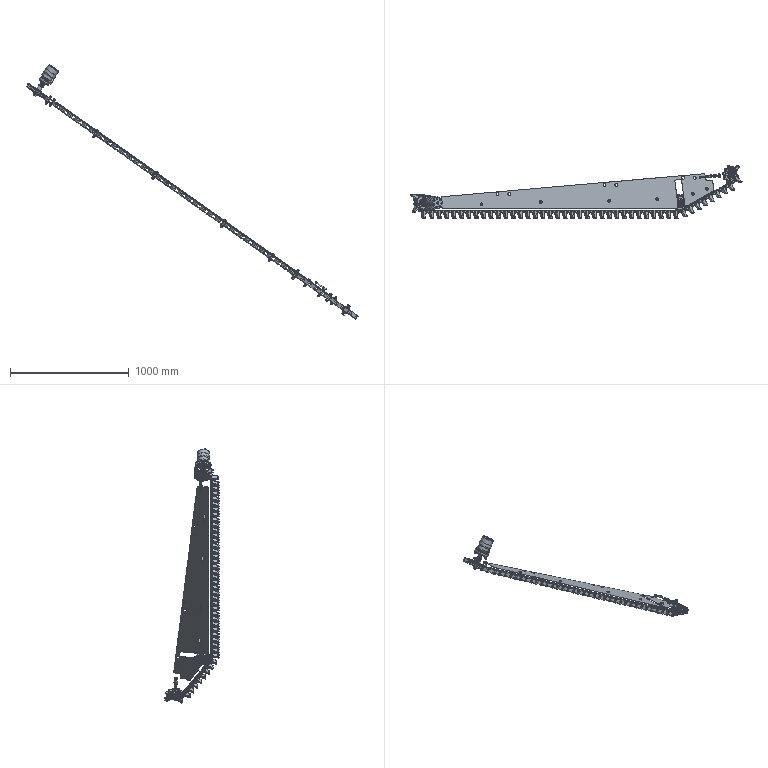Part | STEP file | COMPOUND | 189 solids | 4063 faces | volume 3878446 mm3 | plane 1975 | cylinder 1545 | cone 442 | torus 94 | spline 6 | sphere 1 | commonest cylinder face diameters 6 x380 18 x380 20 x149 12 x115 4 x95 16 x77